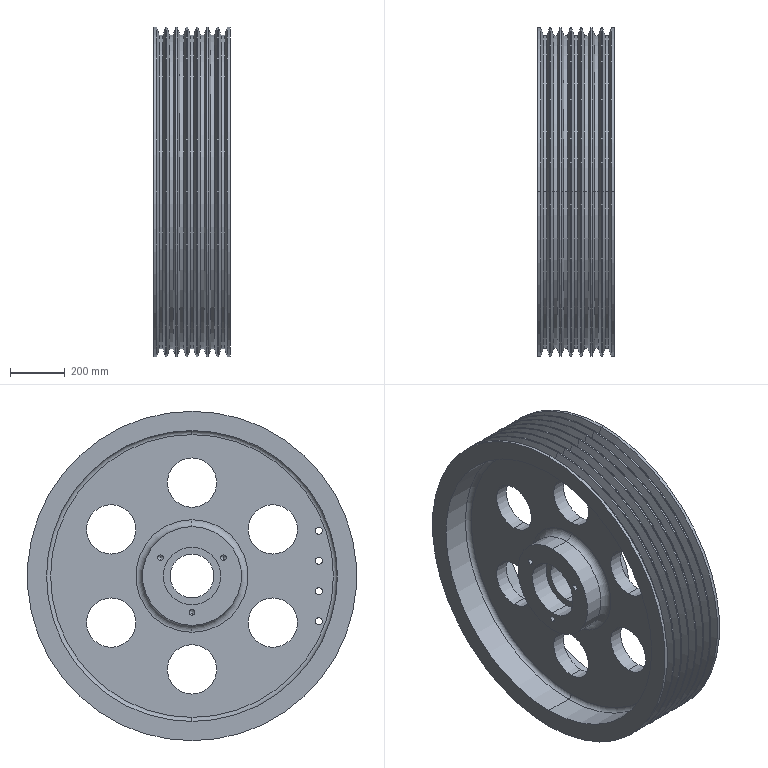Part | SolidWorks | features CirPattern 2, ICE 2, 3DProfileFeature 1, HoleWzd 1, LPattern 1, RevCut 1, Revolution 1 | 1 solid | 117 faces | box 280 x 1200 x 1200 mm | volume 100101767 mm3 | cylinder 68 | cone 34 | torus 8 | plane 7 | commonest cylinder face diameters 1200 x16 1143 x14 180 x12 25 x8 21 x6 1060 x4